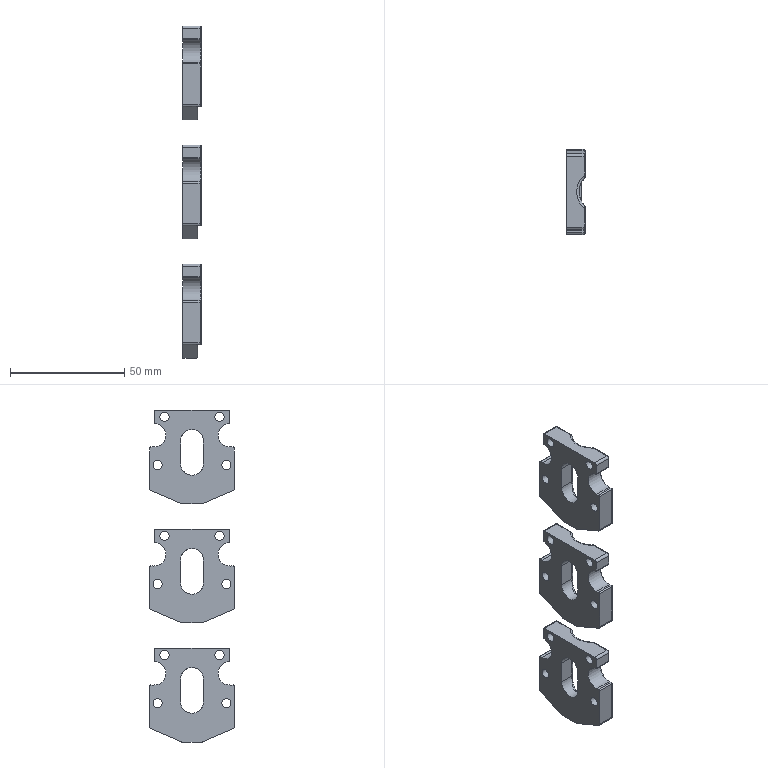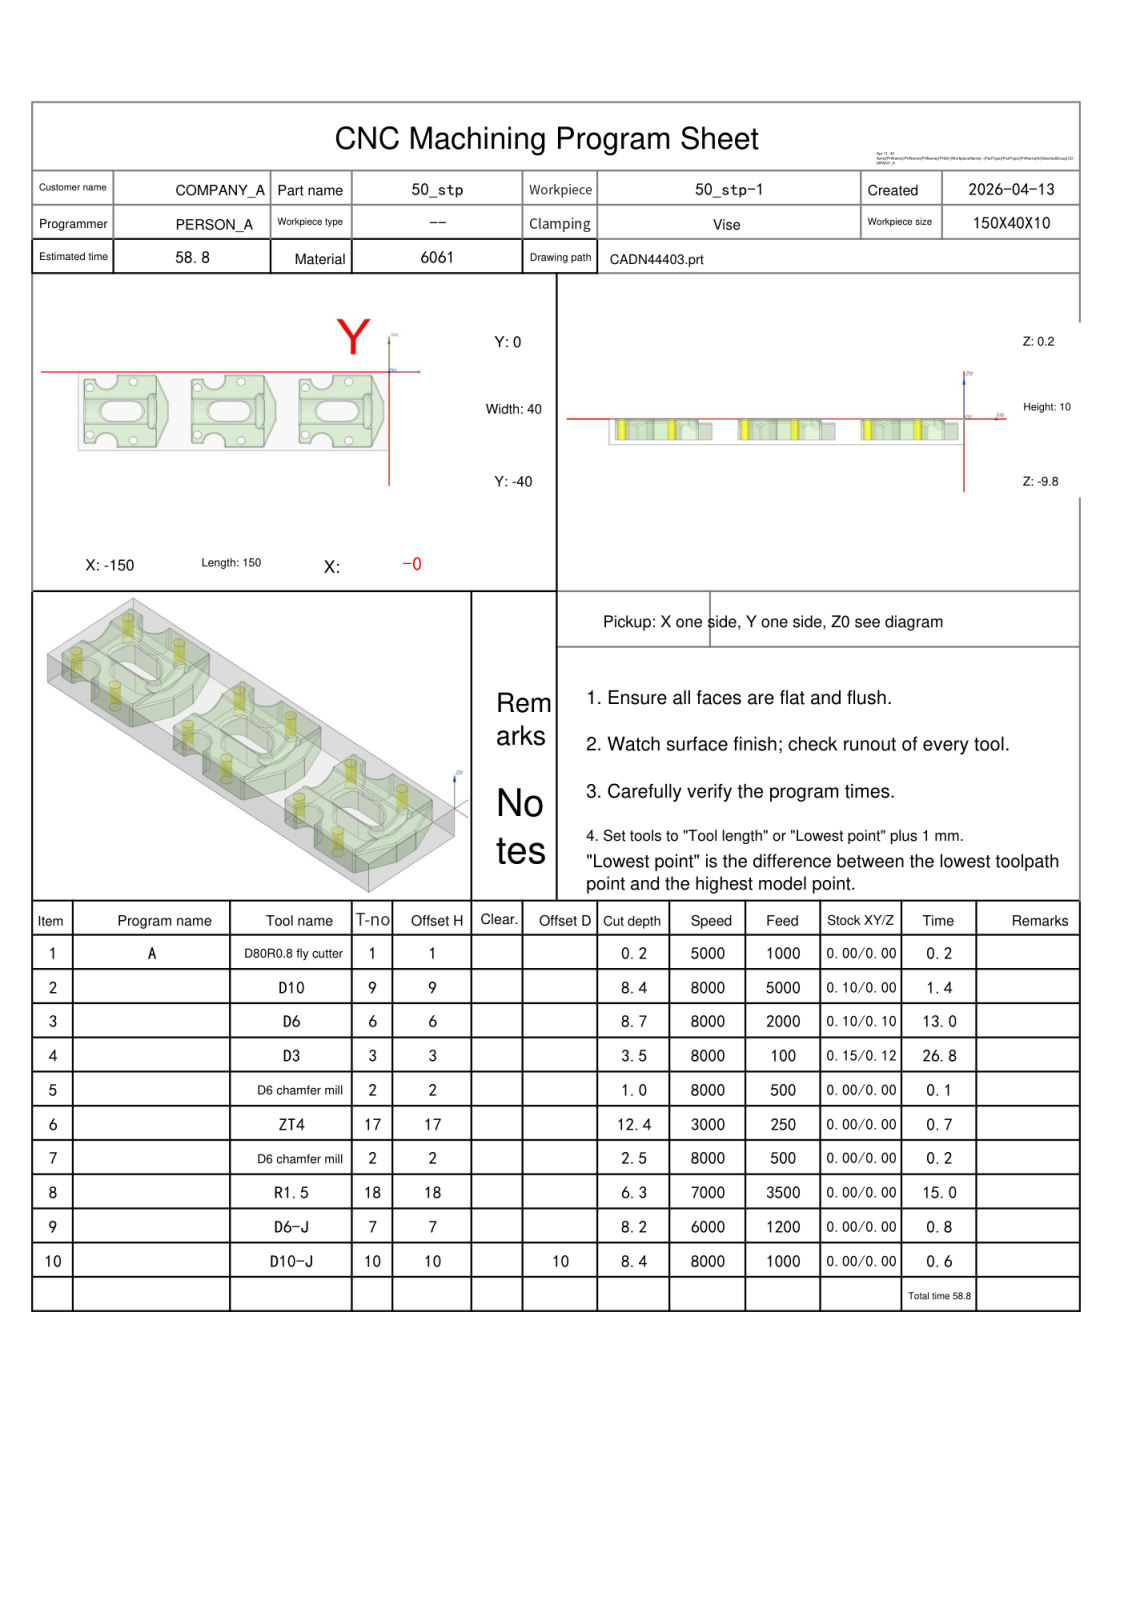NC program | NX | posted by the shop | part box 8 x 37 x 145 mm
Lines 18600 to 18671 of 223411:
N5 T02 M06
(D6 chamfer mill  D=6. R=0. H=02 ce=0.00 di=0.12)
G00 G90 G54 X-40.5 Y-32. M03 S8000
G43 H02 Z20.
M08
G98 G81 X-40.5 Y-32. Z-.8 R1. F500.
X-19.5 Y-35.
Y-5.
X-40.5 Y-8.
X-71.5 Y-5.
X-92.5 Y-8.
X-123.5 Y-5.
X-144.5 Y-8.
Y-32.
X-123.5 Y-35.
X-92.5 Y-32.
X-71.5 Y-35.
G80
G00 Z20.
G91 G28 Z0.0
M05
M09
G91 G28 Z0.0
M01
N6 T17 M06
(ZT4 D=4. DR_a=118 H=17)
G00 G90 G54 X-40.5 Y-32. M03 S3000
G43 H17 Z20.
M08
G98 G83 X-40.5 Y-32. Z-12.202 R1. F250. Q2.
X-19.5 Y-35.
Y-5.
X-40.5 Y-8.
X-71.5 Y-5.
X-92.5 Y-8.
X-123.5 Y-5.
X-144.5 Y-8.
Y-32.
X-123.5 Y-35.
X-92.5 Y-32.
X-71.5 Y-35.
G80
G00 Z20.
G91 G28 Z0.0
M05
M09
G91 G28 Z0.0
M01
N7 T02 M06
(D6 chamfer mill  D=6. R=0. H=02 ce=0.00 di=0.12)
G00 G90 G54 X-40.5 Y-32. M03 S8000
G43 H02 Z20.
M08
G98 G81 X-40.5 Y-32. Z-2.3 R3. F500.
X-19.5 Y-35.
Y-5.
X-40.5 Y-8.
X-71.5 Y-5.
X-92.5 Y-8.
X-123.5 Y-5.
X-144.5 Y-8.
Y-32.
X-123.5 Y-35.
X-92.5 Y-32.
X-71.5 Y-35.
G80
G00 Z20.
G91 G28 Z0.0
M05
M09
G91 G28 Z0.0
M01